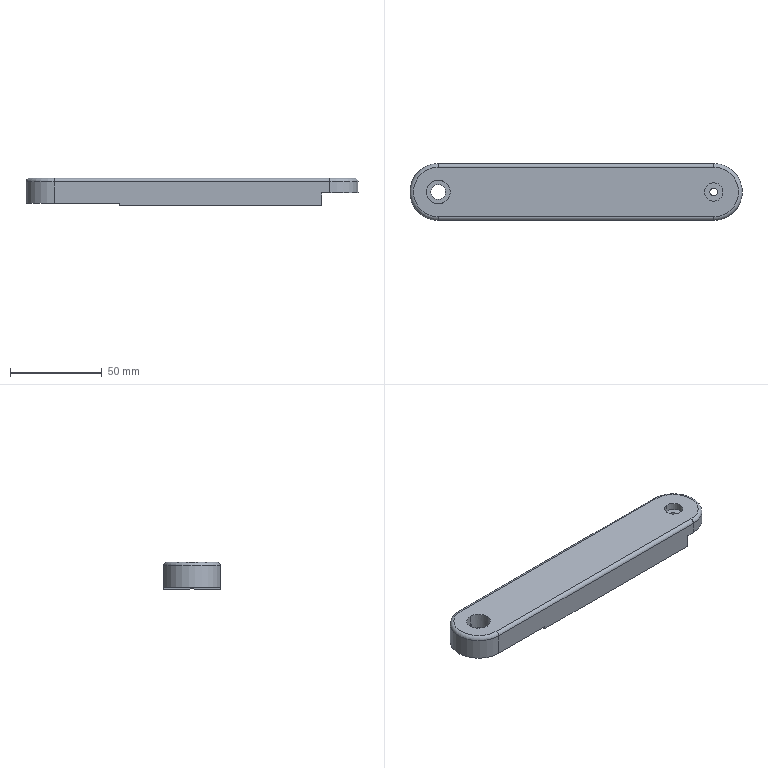NC program | NX | posted with a generic post | part box 181 x 31 x 15 mm
Whole program:
N10 G17 G21 G94 G90
(FLOOR_WALL_COPY_COPY , TOOL : D80)
N12 T19 M6
N14 G54
N16 G17 G0 G90 X-135.5 Y0. S6500 M3
N18 G43 Z30. H19
N20 Z7.
N22 G94 G1 Z4. F1500.
N24 X-130.5
N26 X130.5
N28 X135.5
N30 Z7.
N32 G0 Z30.
N34 X-135.5
N36 Z6.
N38 G1 Z3.
N40 X-130.5
N42 X130.5
N44 X135.5
N46 Z6.
N48 G0 Z30.
N50 X-135.5
N52 Z5.
N54 G1 Z2.
N56 X-130.5
N58 X130.5
N60 X135.5
N62 Z5.
N64 G0 Z30.
N66 X-135.5
N68 Z4.
N70 G1 Z1.
N72 X-130.5
N74 X130.5
N76 X135.5
N78 Z4.
N80 G0 Z30.
N82 X-135.5
N84 Z3.
N86 G1 Z0.
N88 X-130.5
N90 X130.5
N92 X135.5
N94 Z3.
N96 G0 Z30.
N98 M5
(HOLE_MILLING_COPY_1 , TOOL : D6)
N100 T12 M6
N102 G54
N104 G17 G0 G90 X-75. Y0. S9500 M3
N106 G43 Z30. H12
N108 Z0.5
N110 G94 G3 X-73.3 Y-1.7 R1.7 F1650.
N112 X-71.6 Y0. R1.7
N114 X-71.6 Y0. Z0. I-3.4 J0.
N116 X-71.6 Y0. Z-0.5 I-3.4 J0.
N118 X-71.6 Y0. Z-1. I-3.4 J0.
N120 X-71.6 Y0. Z-1.5 I-3.4 J0.
N122 X-71.6 Y0. Z-2. I-3.4 J0.
N124 X-71.6 Y0. Z-2.5 I-3.4 J0.
N126 X-71.6 Y0. Z-3. I-3.4 J0.
N128 X-71.6 Y0. Z-3.5 I-3.4 J0.
N130 X-71.6 Y0. Z-4. I-3.4 J0.
N132 X-71.6 Y0. Z-4.5 I-3.4 J0.
N134 X-71.6 Y0. Z-5. I-3.4 J0.
N136 X-71.6 Y0. Z-5.5 I-3.4 J0.
N138 X-71.6 Y0. Z-6. I-3.4 J0.
N140 X-71.6 Y0. Z-6.5 I-3.4 J0.
N142 X-71.6 Y0. Z-7. I-3.4 J0.
N144 X-71.6 Y0. Z-7.5 I-3.4 J0.
N146 X-71.6 Y0. Z-8. I-3.4 J0.
N148 X-71.6 Y0. Z-8.5 I-3.4 J0.
N150 X-71.6 Y0. Z-9. I-3.4 J0.
N152 X-75. Y3.4 R3.4
N154 X-71.6 Y0. R-3.4
N156 X-73.3 Y1.7 R1.7
N158 X-75. Y0. R1.7
N160 G0 Z30.
N162 M5
(HOLE_MILLING_COPY_COPY , TOOL : D4)
N164 T11 M6
N166 G54
N168 G17 G0 G90 X75. Y0. S9500 M3
N170 G43 Z30. H11
N172 Z0.5
N174 G94 G3 X75.75 Y-0.75 R0.75 F1650.
N176 X76.5 Y0. R0.75
N178 X76.5 Y0. Z0.2 I-1.5 J0.
N180 X76.5 Y0. Z-0.1 I-1.5 J0.
N182 X76.5 Y0. Z-0.4 I-1.5 J0.
N184 X76.5 Y0. Z-0.7 I-1.5 J0.
N186 X76.5 Y0. Z-1. I-1.5 J0.
N188 X76.5 Y0. Z-1.3 I-1.5 J0.
N190 X76.5 Y0. Z-1.6 I-1.5 J0.
N192 X76.5 Y0. Z-1.9 I-1.5 J0.
N194 X76.5 Y0. Z-2.2 I-1.5 J0.
N196 X76.5 Y0. Z-2.5 I-1.5 J0.
N198 X76.5 Y0. Z-2.8 I-1.5 J0.
N200 X76.5 Y0. Z-3.1 I-1.5 J0.
N202 X76.5 Y0. Z-3.4 I-1.5 J0.
N204 X76.5 Y0. Z-3.7 I-1.5 J0.
N206 X76.5 Y0. Z-4. I-1.5 J0.
N208 X75. Y1.5 R1.5
N210 X76.5 Y0. R-1.5
N212 X75.75 Y0.75 R0.75
N214 X75. Y0. R0.75
N216 G0 Z0.5
N218 G3 X76.5 Y-1.5 R1.5
N220 X78. Y0. R1.5
N222 X78. Y0. Z0.2 I-3. J0.
N224 X78. Y0. Z-0.1 I-3. J0.
N226 X78. Y0. Z-0.4 I-3. J0.
N228 X78. Y0. Z-0.7 I-3. J0.
N230 X78. Y0. Z-1. I-3. J0.
N232 X78. Y0. Z-1.3 I-3. J0.
N234 X78. Y0. Z-1.6 I-3. J0.
N236 X78. Y0. Z-1.9 I-3. J0.
N238 X78. Y0. Z-2.2 I-3. J0.
N240 X78. Y0. Z-2.5 I-3. J0.
N242 X78. Y0. Z-2.8 I-3. J0.
N244 X78. Y0. Z-3.1 I-3. J0.
N246 X78. Y0. Z-3.4 I-3. J0.
N248 X78. Y0. Z-3.7 I-3. J0.
N250 X78. Y0. Z-4. I-3. J0.
N252 X75. Y3. R3.
N254 X78. Y0. R-3.
N256 X76.5 Y1.5 R1.5
N258 X75. Y0. R1.5
N260 G0 Z30.
N262 M5
(PLANAR_MILL_COPY_COPY_COPY_COPY_COPY_COPY_1_COPY_1_COPY_1 , TOOL : D6A45)
N264 T01 M6
N266 G54
N268 G17 G0 G90 X73.497 Y-2.596 S9500 M3
N270 G43 Z30. H1
N272 Z0.5
N274 G94 G1 Z-1. F1250.
N276 X74.134 Y-3.7
N278 G3 X75. Y-4.2 R1.
N280 X79.2 Y0. R4.2
N282 X75. Y-4.2 R-4.2
N284 X75.866 Y-3.7 R1.
N286 G1 X76.503 Y-2.596
N288 Z0.5
N290 G0 Z30.
N292 X-76.399 Y-4.277
N294 Z0.5
N296 G1 Z-1.
N298 X-75.866 Y-5.2
N300 G3 X-75. Y-5.7 R1.
N302 X-69.3 Y0. R5.7
N304 X-75. Y-5.7 R-5.7
N306 X-74.134 Y-5.2 R1.
N308 G1 X-73.601 Y-4.277
N310 Z0.5
N312 G0 Z30.
N314 M5
(ZLEVEL_PROFILE_1 , TOOL : D6R0.5)
N316 T18 M6
N318 G54
N320 G17 G0 G90 X3. Y-19.211 S9500 M3
N322 G43 Z30. H18
N324 Z2.991
N326 G94 G1 Z-0.009 F3500.
N328 G3 X0. Y-16.211 R3.
N330 G1 X-75.
N332 G2 X-91.211 Y0. R16.211
N334 X-75. Y16.211 R16.211
N336 G1 X75.
N338 G2 X91.211 Y0. R16.211
N340 X75. Y-16.211 R16.211
N342 G1 X0.
N344 Y-16.275 Z-0.015
N346 Y-16.326 Z-0.021
N348 X75.
N350 G3 X91.326 Y0. R16.326
N352 X75. Y16.326 R16.326
N354 G1 X-75.
N356 G3 X-91.326 Y0. R16.326
N358 X-75. Y-16.326 R16.326
N360 G1 X0.
N362 Y-16.383 Z-0.03
N364 Y-16.433 Z-0.038
N366 X-75.
N368 G2 X-91.433 Y0. R16.433
N370 X-75. Y16.433 R16.433
N372 G1 X75.
N374 G2 X91.433 Y0. R16.433
N376 X75. Y-16.433 R16.433
N378 G1 X0.
N380 Y-16.487 Z-0.048
N382 Y-16.536 Z-0.058
N384 X75.
N386 G3 X91.536 Y0. R16.536
N388 X75. Y16.536 R16.536
N390 G1 X-75.
N392 G3 X-91.536 Y0. R16.536
N394 X-75. Y-16.536 R16.536
N396 G1 X0.
N398 Y-16.589 Z-0.07
N400 Y-16.637 Z-0.082
N402 X-75.
N404 G2 X-91.637 Y0. R16.637
N406 X-75. Y16.637 R16.637
N408 G1 X75.
N410 G2 X91.637 Y0. R16.637
N412 X75. Y-16.637 R16.637
N414 G1 X0.
N416 Y-16.688 Z-0.096
N418 Y-16.735 Z-0.111
N420 X75.
N422 G3 X91.735 Y0. R16.735
N424 X75. Y16.735 R16.735
N426 G1 X-75.
N428 G3 X-91.735 Y0. R16.735
N430 X-75. Y-16.735 R16.735
N432 G1 X0.
N434 Y-16.785 Z-0.127
N436 Y-16.832 Z-0.143
N438 X-75.
N440 G2 X-91.832 Y0. R16.832
N442 X-75. Y16.832 R16.832
N444 G1 X75.
N446 G2 X91.832 Y0. R16.832
N448 X75. Y-16.832 R16.832
N450 G1 X0.
N452 Y-16.881 Z-0.16
N454 Y-16.927 Z-0.178
N456 X75.
N458 G3 X91.927 Y0. R16.927
N460 X75. Y16.927 R16.927
N462 G1 X-75.
N464 G3 X-91.927 Y0. R16.927
N466 X-75. Y-16.927 R16.927
N468 G1 X0.
N470 Y-16.975 Z-0.198
N472 Y-17.02 Z-0.218
N474 X-75.
N476 G2 X-92.02 Y0. R17.02
N478 X-75. Y17.02 R17.02
N480 G1 X75.
N482 G2 X92.02 Y0. R17.02
N484 X75. Y-17.02 R17.02
N486 G1 X0.
N488 Y-17.067 Z-0.239
N490 Y-17.112 Z-0.261
N492 X75.
N494 G3 X92.112 Y0. R17.112
N496 X75. Y17.112 R17.112
N498 G1 X-75.
N500 G3 X-92.112 Y0. R17.112
N502 X-75. Y-17.112 R17.112
N504 G1 X0.
N506 Y-17.157 Z-0.284
N508 Y-17.201 Z-0.307
N510 X-75.
N512 G2 X-92.201 Y0. R17.201
N514 X-75. Y17.201 R17.201
N516 G1 X75.
N518 G2 X92.201 Y0. R17.201
N520 X75. Y-17.201 R17.201
N522 G1 X0.
N524 Y-17.246 Z-0.332
N526 Y-17.288 Z-0.357
N528 X75.
N530 G3 X92.288 Y0. R17.288
N532 X75. Y17.288 R17.288
N534 G1 X-75.
N536 G3 X-92.288 Y0. R17.288
N538 X-75. Y-17.288 R17.288
N540 G1 X0.
N542 Y-17.332 Z-0.384
N544 Y-17.373 Z-0.411
N546 X-75.
N548 G2 X-92.373 Y0. R17.373
N550 X-75. Y17.373 R17.373
N552 G1 X75.
N554 G2 X92.373 Y0. R17.373
N556 X75. Y-17.373 R17.373
N558 G1 X0.
N560 Y-17.416 Z-0.439
N562 Y-17.456 Z-0.468
N564 X75.
N566 G3 X92.456 Y0. R17.456
N568 X75. Y17.456 R17.456
N570 G1 X-75.
N572 G3 X-92.456 Y0. R17.456
N574 X-75. Y-17.456 R17.456
N576 G1 X0.
N578 Y-17.497 Z-0.498
N580 Y-17.537 Z-0.528
N582 X-75.
N584 G2 X-92.537 Y0. R17.537
N586 X-75. Y17.537 R17.537
N588 G1 X75.
N590 G2 X92.537 Y0. R17.537
N592 X75. Y-17.537 R17.537
N594 G1 X0.
N596 Y-17.576 Z-0.56
N598 Y-17.615 Z-0.591
N600 X75.
N602 G3 X92.615 Y0. R17.615
N604 X75. Y17.615 R17.615
N606 G1 X-75.
N608 G3 X-92.615 Y0. R17.615
N610 X-75. Y-17.615 R17.615
N612 G1 X0.
N614 Y-17.653 Z-0.624
N616 Y-17.69 Z-0.658
N618 X-75.
N620 G2 X-92.69 Y0. R17.69
N622 X-75. Y17.69 R17.69
N624 G1 X75.
N626 G2 X92.69 Y0. R17.69
N628 X75. Y-17.69 R17.69
N630 G1 X0.
N632 Y-17.727 Z-0.692
N634 Y-17.762 Z-0.727
N636 X75.
N638 G3 X92.762 Y0. R17.762
N640 X75. Y17.762 R17.762
N642 G1 X-75.
N644 G3 X-92.762 Y0. R17.762
N646 X-75. Y-17.762 R17.762
N648 G1 X0.
N650 Y-17.798 Z-0.763
N652 Y-17.832 Z-0.799
N654 X-75.
N656 G2 X-92.832 Y0. R17.832
N658 X-75. Y17.832 R17.832
N660 G1 X75.
N662 G2 X92.832 Y0. R17.832
N664 X75. Y-17.832 R17.832
N666 G1 X0.
N668 Y-17.866 Z-0.836
N670 Y-17.899 Z-0.874
N672 X75.
N674 G3 X92.899 Y0. R17.899
N676 X75. Y17.899 R17.899
N678 G1 X-75.
N680 G3 X-92.899 Y0. R17.899
N682 X-75. Y-17.899 R17.899
N684 G1 X0.
N686 Y-17.931 Z-0.912
N688 Y-17.962 Z-0.951
N690 X-75.
N692 G2 X-92.962 Y0. R17.962
N694 X-75. Y17.962 R17.962
N696 G1 X75.
N698 G2 X92.962 Y0. R17.962
N700 X75. Y-17.962 R17.962
N702 G1 X0.
N704 Y-17.993 Z-0.991
N706 Y-18.023 Z-1.031
N708 X75.
N710 G3 X93.023 Y0. R18.023
N712 X75. Y18.023 R18.023
N714 G1 X-75.
N716 G3 X-93.023 Y0. R18.023
N718 X-75. Y-18.023 R18.023
N720 G1 X0.
N722 Y-18.052 Z-1.072
N724 Y-18.08 Z-1.113
N726 X-75.
N728 G2 X-93.08 Y0. R18.08
N730 X-75. Y18.08 R18.08
N732 G1 X75.
N734 G2 X93.08 Y0. R18.08
N736 X75. Y-18.08 R18.08
N738 G1 X0.
N740 Y-18.108 Z-1.155
N742 Y-18.134 Z-1.198
N744 X75.
N746 G3 X93.134 Y0. R18.134
N748 X75. Y18.134 R18.134
N750 G1 X-75.
N752 G3 X-93.134 Y0. R18.134
N754 X-75. Y-18.134 R18.134
N756 G1 X0.
N758 Y-18.16 Z-1.241
N760 Y-18.184 Z-1.284
N762 X-75.
N764 G2 X-93.184 Y0. R18.184
N766 X-75. Y18.184 R18.184
N768 G1 X75.
N770 G2 X93.184 Y0. R18.184
N772 X75. Y-18.184 R18.184
N774 G1 X0.
N776 Y-18.208 Z-1.328
N778 Y-18.231 Z-1.373
N780 X75.
N782 G3 X93.231 Y0. R18.231
N784 X75. Y18.231 R18.231
N786 G1 X-75.
N788 G3 X-93.231 Y0. R18.231
N790 X-75. Y-18.231 R18.231
N792 G1 X0.
N794 Y-18.254 Z-1.418
N796 Y-18.275 Z-1.463
N798 X-75.
N800 G2 X-93.275 Y0. R18.275
N802 X-75. Y18.275 R18.275
N804 G1 X75.
N806 G2 X93.275 Y0. R18.275
N808 X75. Y-18.275 R18.275
N810 G1 X0.
N812 Y-18.295 Z-1.509
N814 Y-18.314 Z-1.555
N816 X75.
N818 G3 X93.314 Y0. R18.314
N820 X75. Y18.314 R18.314
N822 G1 X-75.
N824 G3 X-93.314 Y0. R18.314
N826 X-75. Y-18.314 R18.314
N828 G1 X0.
N830 Y-18.333 Z-1.601
N832 Y-18.35 Z-1.648
N834 X-75.
N836 G2 X-93.35 Y0. R18.35
N838 X-75. Y18.35 R18.35
N840 G1 X75.
N842 G2 X93.35 Y0. R18.35
N844 X75. Y-18.35 R18.35
N846 G1 X0.
N848 Y-18.367 Z-1.695
N850 Y-18.383 Z-1.743
N852 X75.
N854 G3 X93.383 Y0. R18.383
N856 X75. Y18.383 R18.383
N858 G1 X-75.
N860 G3 X-93.383 Y0. R18.383
N862 X-75. Y-18.383 R18.383
N864 G1 X0.
N866 Y-18.397 Z-1.791
N868 Y-18.411 Z-1.839
N870 X-75.
N872 G2 X-93.411 Y0. R18.411
N874 X-75. Y18.411 R18.411
N876 G1 X75.
N878 G2 X93.411 Y0. R18.411
N880 X75. Y-18.411 R18.411
N882 G1 X0.
N884 Y-18.424 Z-1.887
N886 Y-18.435 Z-1.936
N888 X75.
N890 G3 X93.435 Y0. R18.435
N892 X75. Y18.435 R18.435
N894 G1 X-75.
N896 G3 X-93.435 Y0. R18.435
N898 X-75. Y-18.435 R18.435
N900 G1 X0.
N902 Y-18.446 Z-1.985
N904 Y-18.456 Z-2.034
N906 X-75.
N908 G2 X-93.456 Y0. R18.456
N910 X-75. Y18.456 R18.456
N912 G1 X75.
N914 G2 X93.456 Y0. R18.456
N916 X75. Y-18.456 R18.456
N918 G1 X0.
N920 Y-18.465 Z-2.083
N922 Y-18.473 Z-2.132
N924 X75.
N926 G3 X93.473 Y0. R18.473
N928 X75. Y18.473 R18.473
N930 G1 X-75.
N932 G3 X-93.473 Y0. R18.473
N934 X-75. Y-18.473 R18.473
N936 G1 X0.
N938 Y-18.479 Z-2.178
N940 Y-18.485 Z-2.224
N942 X-75.
N944 G2 X-93.485 Y0. R18.485
N946 X-75. Y18.485 R18.485
N948 G1 X75.
N950 G2 X93.485 Y0. R18.485
N952 X75. Y-18.485 R18.485
N954 G1 X0.
N956 Y-18.493 Z-2.316
N958 X75.
N960 G3 X93.493 Y0. R18.493
N962 X75. Y18.493 R18.493
N964 G1 X-75.
N966 G3 X-93.493 Y0. R18.493
N968 X-75. Y-18.493 R18.493
N970 G1 X0.
N972 Y-18.497 Z-2.408
N974 X-75.
N976 X-75.808 Y-18.481
N978 G2 X-75. Y18.498 R18.498
N980 G1 X75.
N982 G2 X75.356 Y-18.495 R18.498
N984 X75.136 Y-18.497 R11.435
N986 G1 X0.
N988 Y-18.498 Z-2.5
N990 X75.
N992 X75.116 Y-18.497
N994 X75.808 Y-18.481
N996 G3 X78.799 Y-18.109 R19.713
N998 X82.559 Y-16.883 R18.855
N1000 G1 X82.731 Y-16.806
N1002 X83.424 Y-16.469
N1004 X83.951 Y-16.188
N1006 X84.427 Y-15.922
N1008 G3 X85.653 Y-15.123 R26.257
N1010 G1 X86.377 Y-14.592
N1012 G3 X89.655 Y-11.289 R18.833
N1014 X93.264 Y-2.934 R18.411
N1016 X93.401 Y-1.899 R16.203
N1018 X75. Y18.5 R18.499
N1020 G1 X-75.
N1022 G3 X-84.654 Y15.784 R18.57
N1024 X-87.744 Y13.415 R19.401
N1026 G1 X-88.27 Y12.89
N1028 X-88.544 Y12.599
N1030 G3 X-89.572 Y11.397 R16.674
N1032 X-90.527 Y10.077 R26.775
N1034 X-91.944 Y7.422 R20.095
N1036 X-92.547 Y5.873 R19.258
N1038 X-93.491 Y0.518 R18.741
N1040 X-93.489 Y-0.518 R20.526
N1042 G1 X-93.494
N1044 G3 X-92.808 Y-5.006 R18.636
N1046 G1 X-92.77 Y-5.144
N1048 X-92.484 Y-6.041
N1050 X-92.423 Y-6.217
N1052 X-92.091 Y-7.077
N1054 X-92.077 Y-7.113
N1056 X-91.693 Y-7.99
N1058 X-91.385 Y-8.586
N1060 X-91.019 Y-9.259
N1062 X-90.693 Y-9.794
N1064 X-90.665 Y-9.838
N1066 G3 X-89.438 Y-11.564 R18.055
N1068 X-88.308 Y-12.863 R23.511
N1070 X-86.136 Y-14.782 R22.388
N1072 X-83.174 Y-16.598 R19.983
N1074 X-80.962 Y-17.527 R23.313
N1076 X-76.5 Y-18.437 R19.439
N1078 G1 X-75.808 Y-18.481
N1080 X-75. Y-18.498
N1082 X0.
N1084 G2 X3. Y-21.498 R3.
N1086 G1 Z0.5
N1088 G0 Z30.
N1090 M5
(刀补12_COPY , TOOL : D6)
N1092 T12 M6
N1094 G54
N1096 G17 G0 G90 X-75. Y0. S9500 M3
N1098 G43 Z30. H12
N1100 Z0.5
N1102 G41 G94 G1 X-74.977 Y-0.399 F1000. D12
N1104 G3 X-71.55 Y0. R1.737
N1106 X-71.55 Y0. Z-1.5 I-3.45 J0.
N1108 X-71.55 Y0. Z-3.5 I-3.45 J0.
N1110 X-71.55 Y0. Z-5.5 I-3.45 J0.
N1112 X-71.55 Y0. Z-7.5 I-3.45 J0.
N1114 X-75. Y-3.45 Z-9. R-3.45
N1116 X-71.55 Y0. R3.45
N1118 X-75. Y-3.45 R-3.45
N1120 X-74.601 Y-0.023 R1.737
N1122 G40
N1124 G1 X-75. Y0.
N1126 G0 Z30.
N1128 M5
N1130 M2